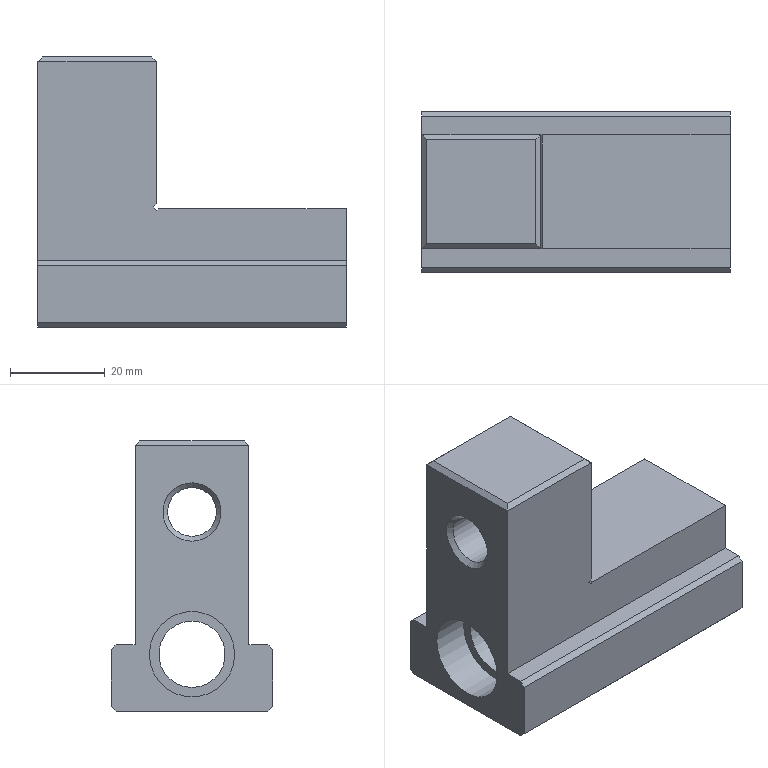Part | NX | features DATUM_CSYS 5, CHAMFER 4, SKETCH 4, BLOCK 3, CYLINDER 2, HOLE PACKAGE 2, SIMPLE HOLE 2, SYMBOLIC_THREAD 2, EXTRUDE 1 | 1 solid | 31 faces | box 65 x 34 x 57 mm | volume 53379 mm3 | plane 25 | cylinder 4 | cone 2 | commonest cylinder face diameters 18 x2 10.3 x1 14 x1
STEP:
#1=CARTESIAN_POINT('',(25.,5.,25.98));
#2=VERTEX_POINT('',#1);
#3=CARTESIAN_POINT('',(25.,5.,56.));
#4=VERTEX_POINT('',#3);
#5=CARTESIAN_POINT('',(25.,5.,0.));
#6=DIRECTION('',(0.,0.,1.));
#7=VECTOR('',#6,1000.);
#8=LINE('',#5,#7);
#9=EDGE_CURVE('',#2,#4,#8,.T.);
#10=ORIENTED_EDGE('',*,*,#9,.T.);
#11=CARTESIAN_POINT('',(0.,5.,56.));
#12=VERTEX_POINT('',#11);
#13=CARTESIAN_POINT('',(12.5,5.,56.));
#14=DIRECTION('',(-1.,0.,0.));
#15=VECTOR('',#14,1000.);
#16=LINE('',#13,#15);
#17=EDGE_CURVE('',#4,#12,#16,.T.);
#18=ORIENTED_EDGE('',*,*,#17,.T.);
#19=CARTESIAN_POINT('',(0.,5.,14.));
#20=VERTEX_POINT('',#19);
#21=CARTESIAN_POINT('',(0.,5.,0.));
#22=DIRECTION('',(0.,0.,1.));
#23=VECTOR('',#22,1000.);
#24=LINE('',#21,#23);
#25=EDGE_CURVE('',#20,#12,#24,.T.);
#26=ORIENTED_EDGE('',*,*,#25,.F.);
#27=CARTESIAN_POINT('',(65.,5.,14.));
#28=VERTEX_POINT('',#27);
#29=CARTESIAN_POINT('',(32.5,5.,14.));
#30=DIRECTION('',(1.,0.,0.));
#31=VECTOR('',#30,1000.);
#32=LINE('',#29,#31);
#33=EDGE_CURVE('',#20,#28,#32,.T.);
#34=ORIENTED_EDGE('',*,*,#33,.T.);
#35=CARTESIAN_POINT('',(65.,5.,25.));
#36=VERTEX_POINT('',#35);
#37=CARTESIAN_POINT('',(65.,5.,14.));
#38=DIRECTION('',(0.,0.,1.));
#39=VECTOR('',#38,1000.);
#40=LINE('',#37,#39);
#41=EDGE_CURVE('',#28,#36,#40,.T.);
#42=ORIENTED_EDGE('',*,*,#41,.T.);
#43=CARTESIAN_POINT('',(25.435,5.,25.));
#44=VERTEX_POINT('',#43);
#45=CARTESIAN_POINT('',(45.,5.,25.));
#46=DIRECTION('',(-1.,0.,0.));
#47=VECTOR('',#46,1000.);
#48=LINE('',#45,#47);
#49=EDGE_CURVE('',#36,#44,#48,.T.);
#50=ORIENTED_EDGE('',*,*,#49,.T.);
#51=CARTESIAN_POINT('',(25.081,5.,24.646));
#52=VERTEX_POINT('',#51);
#53=CARTESIAN_POINT('',(25.435,5.,25.));
#54=DIRECTION('',(-0.7071,0.,-0.7071));
#55=VECTOR('',#54,1000.);
#56=LINE('',#53,#55);
#57=EDGE_CURVE('',#44,#52,#56,.T.);
#58=ORIENTED_EDGE('',*,*,#57,.T.);
#59=CARTESIAN_POINT('',(24.374,5.,25.354));
#60=VERTEX_POINT('',#59);
#61=CARTESIAN_POINT('',(25.081,5.,24.646));
#62=DIRECTION('',(-0.7071,0.,0.7071));
#63=VECTOR('',#62,1000.);
#64=LINE('',#61,#63);
#65=EDGE_CURVE('',#52,#60,#64,.T.);
#66=ORIENTED_EDGE('',*,*,#65,.T.);
#67=CARTESIAN_POINT('',(24.374,5.,25.354));
#68=DIRECTION('',(0.7071,0.,0.7071));
#69=VECTOR('',#68,1000.);
#70=LINE('',#67,#69);
#71=EDGE_CURVE('',#60,#2,#70,.T.);
#72=ORIENTED_EDGE('',*,*,#71,.T.);
#73=EDGE_LOOP('',(#10,#18,#26,#34,#42,#50,#58,#66,#72));
#74=FACE_BOUND('',#73,.T.);
#75=CARTESIAN_POINT('',(12.5,5.,0.));
#76=DIRECTION('',(0.,-1.,0.));
#77=DIRECTION('',(0.,0.,-1.));
#78=AXIS2_PLACEMENT_3D('',#75,#76,#77);
#79=PLANE('',#78);
#80=ADVANCED_FACE('',(#74),#79,.T.);
#81=CARTESIAN_POINT('',(25.,17.,35.85));
#82=VERTEX_POINT('',#81);
#83=CARTESIAN_POINT('',(25.,17.,42.));
#84=DIRECTION('',(1.,0.,0.));
#85=DIRECTION('',(0.,0.,-1.));
#86=AXIS2_PLACEMENT_3D('',#83,#84,#85);
#87=CIRCLE('',#86,6.15);
#88=EDGE_CURVE('',#82,#82,#87,.F.);
#89=ORIENTED_EDGE('',*,*,#88,.T.);
#90=EDGE_LOOP('',(#89));
#91=FACE_BOUND('',#90,.T.);
#92=ORIENTED_EDGE('',*,*,#9,.F.);
#93=CARTESIAN_POINT('',(25.,29.,25.98));
#94=VERTEX_POINT('',#93);
#95=CARTESIAN_POINT('',(25.,29.,25.98));
#96=DIRECTION('',(0.,-1.,0.));
#97=VECTOR('',#96,1000.);
#98=LINE('',#95,#97);
#99=EDGE_CURVE('',#94,#2,#98,.T.);
#100=ORIENTED_EDGE('',*,*,#99,.F.);
#101=CARTESIAN_POINT('',(25.,29.,56.));
#102=VERTEX_POINT('',#101);
#103=CARTESIAN_POINT('',(25.,29.,0.));
#104=DIRECTION('',(0.,0.,1.));
#105=VECTOR('',#104,1000.);
#106=LINE('',#103,#105);
#107=EDGE_CURVE('',#94,#102,#106,.T.);
#108=ORIENTED_EDGE('',*,*,#107,.T.);
#109=CARTESIAN_POINT('',(25.,17.,56.));
#110=DIRECTION('',(0.,-1.,0.));
#111=VECTOR('',#110,1000.);
#112=LINE('',#109,#111);
#113=EDGE_CURVE('',#102,#4,#112,.T.);
#114=ORIENTED_EDGE('',*,*,#113,.T.);
#115=EDGE_LOOP('',(#92,#100,#108,#114));
#116=FACE_BOUND('',#115,.T.);
#117=CARTESIAN_POINT('',(25.,17.,0.));
#118=DIRECTION('',(1.,0.,0.));
#119=DIRECTION('',(0.,0.,-1.));
#120=AXIS2_PLACEMENT_3D('',#117,#118,#119);
#121=PLANE('',#120);
#122=ADVANCED_FACE('',(#91,#116),#121,.T.);
#123=CARTESIAN_POINT('',(25.435,29.,25.));
#124=VERTEX_POINT('',#123);
#125=CARTESIAN_POINT('',(65.,29.,25.));
#126=VERTEX_POINT('',#125);
#127=CARTESIAN_POINT('',(45.,29.,25.));
#128=DIRECTION('',(1.,0.,0.));
#129=VECTOR('',#128,1000.);
#130=LINE('',#127,#129);
#131=EDGE_CURVE('',#124,#126,#130,.T.);
#132=ORIENTED_EDGE('',*,*,#131,.F.);
#133=CARTESIAN_POINT('',(25.435,29.,25.));
#134=DIRECTION('',(0.,-1.,0.));
#135=VECTOR('',#134,1000.);
#136=LINE('',#133,#135);
#137=EDGE_CURVE('',#124,#44,#136,.T.);
#138=ORIENTED_EDGE('',*,*,#137,.T.);
#139=ORIENTED_EDGE('',*,*,#49,.F.);
#140=CARTESIAN_POINT('',(65.,17.,25.));
#141=DIRECTION('',(0.,-1.,0.));
#142=VECTOR('',#141,1000.);
#143=LINE('',#140,#142);
#144=EDGE_CURVE('',#126,#36,#143,.T.);
#145=ORIENTED_EDGE('',*,*,#144,.F.);
#146=EDGE_LOOP('',(#132,#138,#139,#145));
#147=FACE_BOUND('',#146,.T.);
#148=CARTESIAN_POINT('',(45.,17.,25.));
#149=DIRECTION('',(0.,0.,1.));
#150=DIRECTION('',(1.,0.,0.));
#151=AXIS2_PLACEMENT_3D('',#148,#149,#150);
#152=PLANE('',#151);
#153=ADVANCED_FACE('',(#147),#152,.T.);
#154=CARTESIAN_POINT('',(0.,1.,14.));
#155=VERTEX_POINT('',#154);
#156=CARTESIAN_POINT('',(0.,17.,14.));
#157=DIRECTION('',(0.,1.,0.));
#158=VECTOR('',#157,1000.);
#159=LINE('',#156,#158);
#160=EDGE_CURVE('',#155,#20,#159,.T.);
#161=ORIENTED_EDGE('',*,*,#160,.F.);
#162=CARTESIAN_POINT('',(65.,1.,14.));
#163=VERTEX_POINT('',#162);
#164=CARTESIAN_POINT('',(32.5,1.,14.));
#165=DIRECTION('',(1.,0.,0.));
#166=VECTOR('',#165,1000.);
#167=LINE('',#164,#166);
#168=EDGE_CURVE('',#155,#163,#167,.T.);
#169=ORIENTED_EDGE('',*,*,#168,.T.);
#170=CARTESIAN_POINT('',(65.,17.,14.));
#171=DIRECTION('',(0.,-1.,0.));
#172=VECTOR('',#171,1000.);
#173=LINE('',#170,#172);
#174=EDGE_CURVE('',#28,#163,#173,.T.);
#175=ORIENTED_EDGE('',*,*,#174,.F.);
#176=ORIENTED_EDGE('',*,*,#33,.F.);
#177=EDGE_LOOP('',(#161,#169,#175,#176));
#178=FACE_BOUND('',#177,.T.);
#179=CARTESIAN_POINT('',(32.5,17.,14.));
#180=DIRECTION('',(0.,0.,1.));
#181=DIRECTION('',(1.,0.,0.));
#182=AXIS2_PLACEMENT_3D('',#179,#180,#181);
#183=PLANE('',#182);
#184=ADVANCED_FACE('',(#178),#183,.T.);
#185=CARTESIAN_POINT('',(65.,33.,14.));
#186=VERTEX_POINT('',#185);
#187=CARTESIAN_POINT('',(65.,29.,14.));
#188=VERTEX_POINT('',#187);
#189=CARTESIAN_POINT('',(65.,17.,14.));
#190=DIRECTION('',(0.,-1.,0.));
#191=VECTOR('',#190,1000.);
#192=LINE('',#189,#191);
#193=EDGE_CURVE('',#186,#188,#192,.T.);
#194=ORIENTED_EDGE('',*,*,#193,.F.);
#195=CARTESIAN_POINT('',(0.,33.,14.));
#196=VERTEX_POINT('',#195);
#197=CARTESIAN_POINT('',(32.5,33.,14.));
#198=DIRECTION('',(-1.,0.,0.));
#199=VECTOR('',#198,1000.);
#200=LINE('',#197,#199);
#201=EDGE_CURVE('',#186,#196,#200,.T.);
#202=ORIENTED_EDGE('',*,*,#201,.T.);
#203=CARTESIAN_POINT('',(0.,29.,14.));
#204=VERTEX_POINT('',#203);
#205=CARTESIAN_POINT('',(0.,17.,14.));
#206=DIRECTION('',(0.,1.,0.));
#207=VECTOR('',#206,1000.);
#208=LINE('',#205,#207);
#209=EDGE_CURVE('',#204,#196,#208,.T.);
#210=ORIENTED_EDGE('',*,*,#209,.F.);
#211=CARTESIAN_POINT('',(32.5,29.,14.));
#212=DIRECTION('',(-1.,0.,0.));
#213=VECTOR('',#212,1000.);
#214=LINE('',#211,#213);
#215=EDGE_CURVE('',#188,#204,#214,.T.);
#216=ORIENTED_EDGE('',*,*,#215,.F.);
#217=EDGE_LOOP('',(#194,#202,#210,#216));
#218=FACE_BOUND('',#217,.T.);
#219=CARTESIAN_POINT('',(32.5,17.,14.));
#220=DIRECTION('',(0.,0.,1.));
#221=DIRECTION('',(1.,0.,0.));
#222=AXIS2_PLACEMENT_3D('',#219,#220,#221);
#223=PLANE('',#222);
#224=ADVANCED_FACE('',(#218),#223,.T.);
#225=CARTESIAN_POINT('',(65.,0.,1.));
#226=VERTEX_POINT('',#225);
#227=CARTESIAN_POINT('',(65.,0.,13.));
#228=VERTEX_POINT('',#227);
#229=CARTESIAN_POINT('',(65.,0.,0.));
#230=DIRECTION('',(0.,0.,1.));
#231=VECTOR('',#230,1000.);
#232=LINE('',#229,#231);
#233=EDGE_CURVE('',#226,#228,#232,.T.);
#234=ORIENTED_EDGE('',*,*,#233,.T.);
#235=CARTESIAN_POINT('',(0.,0.,13.));
#236=VERTEX_POINT('',#235);
#237=CARTESIAN_POINT('',(32.5,0.,13.));
#238=DIRECTION('',(-1.,0.,0.));
#239=VECTOR('',#238,1000.);
#240=LINE('',#237,#239);
#241=EDGE_CURVE('',#228,#236,#240,.T.);
#242=ORIENTED_EDGE('',*,*,#241,.T.);
#243=CARTESIAN_POINT('',(0.,0.,1.));
#244=VERTEX_POINT('',#243);
#245=CARTESIAN_POINT('',(0.,0.,0.));
#246=DIRECTION('',(0.,0.,1.));
#247=VECTOR('',#246,1000.);
#248=LINE('',#245,#247);
#249=EDGE_CURVE('',#244,#236,#248,.T.);
#250=ORIENTED_EDGE('',*,*,#249,.F.);
#251=CARTESIAN_POINT('',(32.5,0.,1.));
#252=DIRECTION('',(1.,0.,0.));
#253=VECTOR('',#252,1000.);
#254=LINE('',#251,#253);
#255=EDGE_CURVE('',#244,#226,#254,.T.);
#256=ORIENTED_EDGE('',*,*,#255,.T.);
#257=EDGE_LOOP('',(#234,#242,#250,#256));
#258=FACE_BOUND('',#257,.T.);
#259=CARTESIAN_POINT('',(32.5,0.,0.));
#260=DIRECTION('',(0.,-1.,0.));
#261=DIRECTION('',(0.,0.,-1.));
#262=AXIS2_PLACEMENT_3D('',#259,#260,#261);
#263=PLANE('',#262);
#264=ADVANCED_FACE('',(#258),#263,.T.);
#265=CARTESIAN_POINT('',(0.,17.,48.15));
#266=VERTEX_POINT('',#265);
#267=CARTESIAN_POINT('',(0.,17.,42.));
#268=DIRECTION('',(-1.,0.,0.));
#269=DIRECTION('',(0.,0.,1.));
#270=AXIS2_PLACEMENT_3D('',#267,#268,#269);
#271=CIRCLE('',#270,6.15);
#272=EDGE_CURVE('',#266,#266,#271,.F.);
#273=ORIENTED_EDGE('',*,*,#272,.T.);
#274=EDGE_LOOP('',(#273));
#275=FACE_BOUND('',#274,.T.);
#276=CARTESIAN_POINT('',(0.,26.,12.));
#277=VERTEX_POINT('',#276);
#278=CARTESIAN_POINT('',(0.,17.,12.));
#279=DIRECTION('',(1.,0.,0.));
#280=DIRECTION('',(0.,1.,0.));
#281=AXIS2_PLACEMENT_3D('',#278,#279,#280);
#282=CIRCLE('',#281,9.);
#283=EDGE_CURVE('',#277,#277,#282,.T.);
#284=ORIENTED_EDGE('',*,*,#283,.T.);
#285=EDGE_LOOP('',(#284));
#286=FACE_BOUND('',#285,.T.);
#287=CARTESIAN_POINT('',(0.,34.,1.));
#288=VERTEX_POINT('',#287);
#289=CARTESIAN_POINT('',(0.,34.,13.));
#290=VERTEX_POINT('',#289);
#291=CARTESIAN_POINT('',(0.,34.,0.));
#292=DIRECTION('',(0.,0.,1.));
#293=VECTOR('',#292,1000.);
#294=LINE('',#291,#293);
#295=EDGE_CURVE('',#288,#290,#294,.T.);
#296=ORIENTED_EDGE('',*,*,#295,.F.);
#297=CARTESIAN_POINT('',(0.,33.,0.));
#298=VERTEX_POINT('',#297);
#299=CARTESIAN_POINT('',(0.,25.,-8.));
#300=DIRECTION('',(0.,0.7071,0.7071));
#301=VECTOR('',#300,1000.);
#302=LINE('',#299,#301);
#303=EDGE_CURVE('',#288,#298,#302,.F.);
#304=ORIENTED_EDGE('',*,*,#303,.T.);
#305=CARTESIAN_POINT('',(0.,1.,0.));
#306=VERTEX_POINT('',#305);
#307=CARTESIAN_POINT('',(0.,17.,0.));
#308=DIRECTION('',(0.,-1.,0.));
#309=VECTOR('',#308,1000.);
#310=LINE('',#307,#309);
#311=EDGE_CURVE('',#298,#306,#310,.T.);
#312=ORIENTED_EDGE('',*,*,#311,.T.);
#313=CARTESIAN_POINT('',(0.,9.,-8.));
#314=DIRECTION('',(0.,0.7071,-0.7071));
#315=VECTOR('',#314,1000.);
#316=LINE('',#313,#315);
#317=EDGE_CURVE('',#306,#244,#316,.F.);
#318=ORIENTED_EDGE('',*,*,#317,.T.);
#319=ORIENTED_EDGE('',*,*,#249,.T.);
#320=CARTESIAN_POINT('',(0.,2.,15.));
#321=DIRECTION('',(0.,-0.7071,-0.7071));
#322=VECTOR('',#321,1000.);
#323=LINE('',#320,#322);
#324=EDGE_CURVE('',#236,#155,#323,.F.);
#325=ORIENTED_EDGE('',*,*,#324,.T.);
#326=ORIENTED_EDGE('',*,*,#160,.T.);
#327=ORIENTED_EDGE('',*,*,#25,.T.);
#328=CARTESIAN_POINT('',(0.,29.,56.));
#329=VERTEX_POINT('',#328);
#330=CARTESIAN_POINT('',(0.,17.,56.));
#331=DIRECTION('',(0.,1.,0.));
#332=VECTOR('',#331,1000.);
#333=LINE('',#330,#332);
#334=EDGE_CURVE('',#12,#329,#333,.T.);
#335=ORIENTED_EDGE('',*,*,#334,.T.);
#336=CARTESIAN_POINT('',(0.,29.,0.));
#337=DIRECTION('',(0.,0.,1.));
#338=VECTOR('',#337,1000.);
#339=LINE('',#336,#338);
#340=EDGE_CURVE('',#204,#329,#339,.T.);
#341=ORIENTED_EDGE('',*,*,#340,.F.);
#342=ORIENTED_EDGE('',*,*,#209,.T.);
#343=CARTESIAN_POINT('',(0.,32.,15.));
#344=DIRECTION('',(0.,-0.7071,0.7071));
#345=VECTOR('',#344,1000.);
#346=LINE('',#343,#345);
#347=EDGE_CURVE('',#196,#290,#346,.F.);
#348=ORIENTED_EDGE('',*,*,#347,.T.);
#349=EDGE_LOOP('',(#296,#304,#312,#318,#319,#325,#326,#327,#335,#341,#342,#348));
#350=FACE_BOUND('',#349,.T.);
#351=CARTESIAN_POINT('',(0.,17.,0.));
#352=DIRECTION('',(-1.,0.,0.));
#353=DIRECTION('',(0.,0.,1.));
#354=AXIS2_PLACEMENT_3D('',#351,#352,#353);
#355=PLANE('',#354);
#356=ADVANCED_FACE('',(#275,#286,#350),#355,.T.);
#357=CARTESIAN_POINT('',(65.,34.,1.));
#358=VERTEX_POINT('',#357);
#359=CARTESIAN_POINT('',(65.,34.,13.));
#360=VERTEX_POINT('',#359);
#361=CARTESIAN_POINT('',(65.,34.,0.));
#362=DIRECTION('',(0.,0.,1.));
#363=VECTOR('',#362,1000.);
#364=LINE('',#361,#363);
#365=EDGE_CURVE('',#358,#360,#364,.T.);
#366=ORIENTED_EDGE('',*,*,#365,.F.);
#367=CARTESIAN_POINT('',(32.5,34.,1.));
#368=DIRECTION('',(-1.,0.,0.));
#369=VECTOR('',#368,1000.);
#370=LINE('',#367,#369);
#371=EDGE_CURVE('',#358,#288,#370,.T.);
#372=ORIENTED_EDGE('',*,*,#371,.T.);
#373=ORIENTED_EDGE('',*,*,#295,.T.);
#374=CARTESIAN_POINT('',(32.5,34.,13.));
#375=DIRECTION('',(1.,0.,0.));
#376=VECTOR('',#375,1000.);
#377=LINE('',#374,#376);
#378=EDGE_CURVE('',#290,#360,#377,.T.);
#379=ORIENTED_EDGE('',*,*,#378,.T.);
#380=EDGE_LOOP('',(#366,#372,#373,#379));
#381=FACE_BOUND('',#380,.T.);
#382=CARTESIAN_POINT('',(32.5,34.,0.));
#383=DIRECTION('',(0.,1.,0.));
#384=DIRECTION('',(0.,0.,1.));
#385=AXIS2_PLACEMENT_3D('',#382,#383,#384);
#386=PLANE('',#385);
#387=ADVANCED_FACE('',(#381),#386,.T.);
#388=ORIENTED_EDGE('',*,*,#311,.F.);
#389=CARTESIAN_POINT('',(65.,33.,0.));
#390=VERTEX_POINT('',#389);
#391=CARTESIAN_POINT('',(32.5,33.,0.));
#392=DIRECTION('',(1.,0.,0.));
#393=VECTOR('',#392,1000.);
#394=LINE('',#391,#393);
#395=EDGE_CURVE('',#298,#390,#394,.T.);
#396=ORIENTED_EDGE('',*,*,#395,.T.);
#397=CARTESIAN_POINT('',(65.,1.,0.));
#398=VERTEX_POINT('',#397);
#399=CARTESIAN_POINT('',(65.,17.,0.));
#400=DIRECTION('',(0.,1.,0.));
#401=VECTOR('',#400,1000.);
#402=LINE('',#399,#401);
#403=EDGE_CURVE('',#398,#390,#402,.T.);
#404=ORIENTED_EDGE('',*,*,#403,.F.);
#405=CARTESIAN_POINT('',(32.5,1.,0.));
#406=DIRECTION('',(-1.,0.,0.));
#407=VECTOR('',#406,1000.);
#408=LINE('',#405,#407);
#409=EDGE_CURVE('',#398,#306,#408,.T.);
#410=ORIENTED_EDGE('',*,*,#409,.T.);
#411=EDGE_LOOP('',(#388,#396,#404,#410));
#412=FACE_BOUND('',#411,.T.);
#413=CARTESIAN_POINT('',(32.5,17.,0.));
#414=DIRECTION('',(0.,0.,-1.));
#415=DIRECTION('',(-1.,0.,0.));
#416=AXIS2_PLACEMENT_3D('',#413,#414,#415);
#417=PLANE('',#416);
#418=ADVANCED_FACE('',(#412),#417,.T.);
#419=CARTESIAN_POINT('',(65.,8.,12.));
#420=VERTEX_POINT('',#419);
#421=CARTESIAN_POINT('',(65.,17.,12.));
#422=DIRECTION('',(-1.,0.,0.));
#423=DIRECTION('',(0.,-1.,0.));
#424=AXIS2_PLACEMENT_3D('',#421,#422,#423);
#425=CIRCLE('',#424,9.);
#426=EDGE_CURVE('',#420,#420,#425,.T.);
#427=ORIENTED_EDGE('',*,*,#426,.T.);
#428=EDGE_LOOP('',(#427));
#429=FACE_BOUND('',#428,.T.);
#430=ORIENTED_EDGE('',*,*,#403,.T.);
#431=CARTESIAN_POINT('',(65.,25.,-8.));
#432=DIRECTION('',(0.,-0.7071,-0.7071));
#433=VECTOR('',#432,1000.);
#434=LINE('',#431,#433);
#435=EDGE_CURVE('',#390,#358,#434,.F.);
#436=ORIENTED_EDGE('',*,*,#435,.T.);
#437=ORIENTED_EDGE('',*,*,#365,.T.);
#438=CARTESIAN_POINT('',(65.,32.,15.));
#439=DIRECTION('',(0.,0.7071,-0.7071));
#440=VECTOR('',#439,1000.);
#441=LINE('',#438,#440);
#442=EDGE_CURVE('',#360,#186,#441,.F.);
#443=ORIENTED_EDGE('',*,*,#442,.T.);
#444=ORIENTED_EDGE('',*,*,#193,.T.);
#445=CARTESIAN_POINT('',(65.,29.,14.));
#446=DIRECTION('',(0.,0.,1.));
#447=VECTOR('',#446,1000.);
#448=LINE('',#445,#447);
#449=EDGE_CURVE('',#188,#126,#448,.T.);
#450=ORIENTED_EDGE('',*,*,#449,.T.);
#451=ORIENTED_EDGE('',*,*,#144,.T.);
#452=ORIENTED_EDGE('',*,*,#41,.F.);
#453=ORIENTED_EDGE('',*,*,#174,.T.);
#454=CARTESIAN_POINT('',(65.,2.,15.));
#455=DIRECTION('',(0.,0.7071,0.7071));
#456=VECTOR('',#455,1000.);
#457=LINE('',#454,#456);
#458=EDGE_CURVE('',#163,#228,#457,.F.);
#459=ORIENTED_EDGE('',*,*,#458,.T.);
#460=ORIENTED_EDGE('',*,*,#233,.F.);
#461=CARTESIAN_POINT('',(65.,9.,-8.));
#462=DIRECTION('',(0.,-0.7071,0.7071));
#463=VECTOR('',#462,1000.);
#464=LINE('',#461,#463);
#465=EDGE_CURVE('',#226,#398,#464,.F.);
#466=ORIENTED_EDGE('',*,*,#465,.T.);
#467=EDGE_LOOP('',(#430,#436,#437,#443,#444,#450,#451,#452,#453,#459,#460,#466));
#468=FACE_BOUND('',#467,.T.);
#469=CARTESIAN_POINT('',(65.,17.,0.));
#470=DIRECTION('',(1.,0.,0.));
#471=DIRECTION('',(0.,0.,-1.));
#472=AXIS2_PLACEMENT_3D('',#469,#470,#471);
#473=PLANE('',#472);
#474=ADVANCED_FACE('',(#429,#468),#473,.T.);
#475=CARTESIAN_POINT('',(24.,6.,57.));
#476=VERTEX_POINT('',#475);
#477=CARTESIAN_POINT('',(24.,28.,57.));
#478=VERTEX_POINT('',#477);
#479=CARTESIAN_POINT('',(24.,17.,57.));
#480=DIRECTION('',(0.,1.,0.));
#481=VECTOR('',#480,1000.);
#482=LINE('',#479,#481);
#483=EDGE_CURVE('',#476,#478,#482,.T.);
#484=ORIENTED_EDGE('',*,*,#483,.T.);
#485=CARTESIAN_POINT('',(1.,28.,57.));
#486=VERTEX_POINT('',#485);
#487=CARTESIAN_POINT('',(12.5,28.,57.));
#488=DIRECTION('',(-1.,0.,0.));
#489=VECTOR('',#488,1000.);
#490=LINE('',#487,#489);
#491=EDGE_CURVE('',#478,#486,#490,.T.);
#492=ORIENTED_EDGE('',*,*,#491,.T.);
#493=CARTESIAN_POINT('',(1.,6.,57.));
#494=VERTEX_POINT('',#493);
#495=CARTESIAN_POINT('',(1.,17.,57.));
#496=DIRECTION('',(0.,-1.,0.));
#497=VECTOR('',#496,1000.);
#498=LINE('',#495,#497);
#499=EDGE_CURVE('',#486,#494,#498,.T.);
#500=ORIENTED_EDGE('',*,*,#499,.T.);
#501=CARTESIAN_POINT('',(12.5,6.,57.));
#502=DIRECTION('',(1.,0.,0.));
#503=VECTOR('',#502,1000.);
#504=LINE('',#501,#503);
#505=EDGE_CURVE('',#494,#476,#504,.T.);
#506=ORIENTED_EDGE('',*,*,#505,.T.);
#507=EDGE_LOOP('',(#484,#492,#500,#506));
#508=FACE_BOUND('',#507,.T.);
#509=CARTESIAN_POINT('',(12.5,17.,57.));
#510=DIRECTION('',(0.,0.,1.));
#511=DIRECTION('',(1.,0.,0.));
#512=AXIS2_PLACEMENT_3D('',#509,#510,#511);
#513=PLANE('',#512);
#514=ADVANCED_FACE('',(#508),#513,.T.);
#515=ORIENTED_EDGE('',*,*,#340,.T.);
#516=CARTESIAN_POINT('',(12.5,29.,56.));
#517=DIRECTION('',(1.,0.,0.));
#518=VECTOR('',#517,1000.);
#519=LINE('',#516,#518);
#520=EDGE_CURVE('',#329,#102,#519,.T.);
#521=ORIENTED_EDGE('',*,*,#520,.T.);
#522=ORIENTED_EDGE('',*,*,#107,.F.);
#523=CARTESIAN_POINT('',(24.374,29.,25.354));
#524=VERTEX_POINT('',#523);
#525=CARTESIAN_POINT('',(24.374,29.,25.354));
#526=DIRECTION('',(0.7071,0.,0.7071));
#527=VECTOR('',#526,1000.);
#528=LINE('',#525,#527);
#529=EDGE_CURVE('',#524,#94,#528,.T.);
#530=ORIENTED_EDGE('',*,*,#529,.F.);
#531=CARTESIAN_POINT('',(25.081,29.,24.646));
#532=VERTEX_POINT('',#531);
#533=CARTESIAN_POINT('',(25.081,29.,24.646));
#534=DIRECTION('',(-0.7071,0.,0.7071));
#535=VECTOR('',#534,1000.);
#536=LINE('',#533,#535);
#537=EDGE_CURVE('',#532,#524,#536,.T.);
#538=ORIENTED_EDGE('',*,*,#537,.F.);
#539=CARTESIAN_POINT('',(25.435,29.,25.));
#540=DIRECTION('',(-0.7071,0.,-0.7071));
#541=VECTOR('',#540,1000.);
#542=LINE('',#539,#541);
#543=EDGE_CURVE('',#124,#532,#542,.T.);
#544=ORIENTED_EDGE('',*,*,#543,.F.);
#545=ORIENTED_EDGE('',*,*,#131,.T.);
#546=ORIENTED_EDGE('',*,*,#449,.F.);
#547=ORIENTED_EDGE('',*,*,#215,.T.);
#548=EDGE_LOOP('',(#515,#521,#522,#530,#538,#544,#545,#546,#547));
#549=FACE_BOUND('',#548,.T.);
#550=CARTESIAN_POINT('',(12.5,29.,0.));
#551=DIRECTION('',(0.,1.,0.));
#552=DIRECTION('',(0.,0.,1.));
#553=AXIS2_PLACEMENT_3D('',#550,#551,#552);
#554=PLANE('',#553);
#555=ADVANCED_FACE('',(#549),#554,.T.);
#556=CARTESIAN_POINT('',(8.,17.,5.));
#557=VERTEX_POINT('',#556);
#558=CARTESIAN_POINT('',(8.,17.,12.));
#559=DIRECTION('',(1.,0.,0.));
#560=DIRECTION('',(0.,0.,-1.));
#561=AXIS2_PLACEMENT_3D('',#558,#559,#560);
#562=CIRCLE('',#561,7.);
#563=EDGE_CURVE('',#557,#557,#562,.T.);
#564=ORIENTED_EDGE('',*,*,#563,.T.);
#565=EDGE_LOOP('',(#564));
#566=FACE_BOUND('',#565,.T.);
#567=CARTESIAN_POINT('',(8.,26.,12.));
#568=VERTEX_POINT('',#567);
#569=CARTESIAN_POINT('',(8.,17.,12.));
#570=DIRECTION('',(-1.,0.,0.));
#571=DIRECTION('',(0.,1.,0.));
#572=AXIS2_PLACEMENT_3D('',#569,#570,#571);
#573=CIRCLE('',#572,9.);
#574=EDGE_CURVE('',#568,#568,#573,.F.);
#575=ORIENTED_EDGE('',*,*,#574,.F.);
#576=EDGE_LOOP('',(#575));
#577=FACE_BOUND('',#576,.T.);
#578=CARTESIAN_POINT('',(8.,17.,12.));
#579=DIRECTION('',(1.,0.,0.));
#580=DIRECTION('',(0.,0.,-1.));
#581=AXIS2_PLACEMENT_3D('',#578,#579,#580);
#582=PLANE('',#581);
#583=ADVANCED_FACE('',(#566,#577),#582,.F.);
#584=ORIENTED_EDGE('',*,*,#574,.T.);
#585=EDGE_LOOP('',(#584));
#586=FACE_BOUND('',#585,.T.);
#587=ORIENTED_EDGE('',*,*,#283,.F.);
#588=EDGE_LOOP('',(#587));
#589=FACE_BOUND('',#588,.T.);
#590=CARTESIAN_POINT('',(0.,17.,12.));
#591=DIRECTION('',(1.,0.,0.));
#592=DIRECTION('',(0.,1.,0.));
#593=AXIS2_PLACEMENT_3D('',#590,#591,#592);
#594=CYLINDRICAL_SURFACE('',#593,9.);
#595=ADVANCED_FACE('',(#586,#589),#594,.F.);
#596=CARTESIAN_POINT('',(57.,17.,5.));
#597=VERTEX_POINT('',#596);
#598=CARTESIAN_POINT('',(57.,17.,12.));
#599=DIRECTION('',(1.,0.,0.));
#600=DIRECTION('',(0.,0.,-1.));
#601=AXIS2_PLACEMENT_3D('',#598,#599,#600);
#602=CIRCLE('',#601,7.);
#603=EDGE_CURVE('',#597,#597,#602,.T.);
#604=ORIENTED_EDGE('',*,*,#603,.F.);
#605=EDGE_LOOP('',(#604));
#606=FACE_BOUND('',#605,.T.);
#607=CARTESIAN_POINT('',(57.,8.,12.));
#608=VERTEX_POINT('',#607);
#609=CARTESIAN_POINT('',(57.,17.,12.));
#610=DIRECTION('',(1.,0.,0.));
#611=DIRECTION('',(0.,-1.,0.));
#612=AXIS2_PLACEMENT_3D('',#609,#610,#611);
#613=CIRCLE('',#612,9.);
#614=EDGE_CURVE('',#608,#608,#613,.F.);
#615=ORIENTED_EDGE('',*,*,#614,.F.);
#616=EDGE_LOOP('',(#615));
#617=FACE_BOUND('',#616,.T.);
#618=CARTESIAN_POINT('',(57.,17.,12.));
#619=DIRECTION('',(-1.,0.,0.));
#620=DIRECTION('',(0.,0.,1.));
#621=AXIS2_PLACEMENT_3D('',#618,#619,#620);
#622=PLANE('',#621);
#623=ADVANCED_FACE('',(#606,#617),#622,.F.);
#624=ORIENTED_EDGE('',*,*,#614,.T.);
#625=EDGE_LOOP('',(#624));
#626=FACE_BOUND('',#625,.T.);
#627=ORIENTED_EDGE('',*,*,#426,.F.);
#628=EDGE_LOOP('',(#627));
#629=FACE_BOUND('',#628,.T.);
#630=CARTESIAN_POINT('',(65.,17.,12.));
#631=DIRECTION('',(-1.,0.,0.));
#632=DIRECTION('',(0.,-1.,0.));
#633=AXIS2_PLACEMENT_3D('',#630,#631,#632);
#634=CYLINDRICAL_SURFACE('',#633,9.);
#635=ADVANCED_FACE('',(#626,#629),#634,.F.);
#636=ORIENTED_EDGE('',*,*,#603,.T.);
#637=EDGE_LOOP('',(#636));
#638=FACE_BOUND('',#637,.T.);
#639=ORIENTED_EDGE('',*,*,#563,.F.);
#640=EDGE_LOOP('',(#639));
#641=FACE_BOUND('',#640,.T.);
#642=CARTESIAN_POINT('',(8.,17.,12.));
#643=DIRECTION('',(1.,0.,0.));
#644=DIRECTION('',(0.,0.,-1.));
#645=AXIS2_PLACEMENT_3D('',#642,#643,#644);
#646=CYLINDRICAL_SURFACE('',#645,7.);
#647=ADVANCED_FACE('',(#638,#641),#646,.F.);
#648=CARTESIAN_POINT('',(24.,17.,36.85));
#649=VERTEX_POINT('',#648);
#650=CARTESIAN_POINT('',(24.,17.,42.));
#651=DIRECTION('',(1.,0.,0.));
#652=DIRECTION('',(0.,0.,-1.));
#653=AXIS2_PLACEMENT_3D('',#650,#651,#652);
#654=CIRCLE('',#653,5.15);
#655=EDGE_CURVE('',#649,#649,#654,.T.);
#656=ORIENTED_EDGE('',*,*,#655,.T.);
#657=EDGE_LOOP('',(#656));
#658=FACE_BOUND('',#657,.T.);
#659=CARTESIAN_POINT('',(1.,17.,47.15));
#660=VERTEX_POINT('',#659);
#661=CARTESIAN_POINT('',(1.,17.,42.));
#662=DIRECTION('',(-1.,0.,0.));
#663=DIRECTION('',(0.,0.,1.));
#664=AXIS2_PLACEMENT_3D('',#661,#662,#663);
#665=CIRCLE('',#664,5.15);
#666=EDGE_CURVE('',#660,#660,#665,.T.);
#667=ORIENTED_EDGE('',*,*,#666,.T.);
#668=EDGE_LOOP('',(#667));
#669=FACE_BOUND('',#668,.T.);
#670=CARTESIAN_POINT('',(0.,17.,42.));
#671=DIRECTION('',(1.,0.,0.));
#672=DIRECTION('',(0.,0.,-1.));
#673=AXIS2_PLACEMENT_3D('',#670,#671,#672);
#674=CYLINDRICAL_SURFACE('',#673,5.15);
#675=ADVANCED_FACE('',(#658,#669),#674,.F.);
#676=ORIENTED_EDGE('',*,*,#499,.F.);
#677=CARTESIAN_POINT('',(4.,25.,60.));
#678=DIRECTION('',(-0.5774,0.5774,-0.5774));
#679=VECTOR('',#678,1000.);
#680=LINE('',#677,#679);
#681=EDGE_CURVE('',#486,#329,#680,.T.);
#682=ORIENTED_EDGE('',*,*,#681,.T.);
#683=ORIENTED_EDGE('',*,*,#334,.F.);
#684=CARTESIAN_POINT('',(4.,9.,60.));
#685=DIRECTION('',(0.5774,0.5774,0.5774));
#686=VECTOR('',#685,1000.);
#687=LINE('',#684,#686);
#688=EDGE_CURVE('',#12,#494,#687,.T.);
#689=ORIENTED_EDGE('',*,*,#688,.T.);
#690=EDGE_LOOP('',(#676,#682,#683,#689));
#691=FACE_BOUND('',#690,.T.);
#692=CARTESIAN_POINT('',(0.,17.,56.));
#693=DIRECTION('',(0.7071,0.,-0.7071));
#694=DIRECTION('',(0.,1.,0.));
#695=AXIS2_PLACEMENT_3D('',#692,#693,#694);
#696=PLANE('',#695);
#697=ADVANCED_FACE('',(#691),#696,.F.);
#698=ORIENTED_EDGE('',*,*,#113,.F.);
#699=CARTESIAN_POINT('',(21.,25.,60.));
#700=DIRECTION('',(-0.5774,-0.5774,0.5774));
#701=VECTOR('',#700,1000.);
#702=LINE('',#699,#701);
#703=EDGE_CURVE('',#102,#478,#702,.T.);
#704=ORIENTED_EDGE('',*,*,#703,.T.);
#705=ORIENTED_EDGE('',*,*,#483,.F.);
#706=CARTESIAN_POINT('',(21.,9.,60.));
#707=DIRECTION('',(0.5774,-0.5774,-0.5774));
#708=VECTOR('',#707,1000.);
#709=LINE('',#706,#708);
#710=EDGE_CURVE('',#476,#4,#709,.T.);
#711=ORIENTED_EDGE('',*,*,#710,.T.);
#712=EDGE_LOOP('',(#698,#704,#705,#711));
#713=FACE_BOUND('',#712,.T.);
#714=CARTESIAN_POINT('',(25.,17.,56.));
#715=DIRECTION('',(-0.7071,0.,-0.7071));
#716=DIRECTION('',(0.,-1.,0.));
#717=AXIS2_PLACEMENT_3D('',#714,#715,#716);
#718=PLANE('',#717);
#719=ADVANCED_FACE('',(#713),#718,.F.);
#720=ORIENTED_EDGE('',*,*,#88,.F.);
#721=EDGE_LOOP('',(#720));
#722=FACE_BOUND('',#721,.T.);
#723=ORIENTED_EDGE('',*,*,#655,.F.);
#724=EDGE_LOOP('',(#723));
#725=FACE_BOUND('',#724,.T.);
#726=CARTESIAN_POINT('',(24.,17.,42.));
#727=DIRECTION('',(1.,0.,0.));
#728=DIRECTION('',(0.,0.,-1.));
#729=AXIS2_PLACEMENT_3D('',#726,#727,#728);
#730=CONICAL_SURFACE('',#729,5.15,0.7854);
#731=ADVANCED_FACE('',(#722,#725),#730,.F.);
#732=ORIENTED_EDGE('',*,*,#666,.F.);
#733=EDGE_LOOP('',(#732));
#734=FACE_BOUND('',#733,.T.);
#735=ORIENTED_EDGE('',*,*,#272,.F.);
#736=EDGE_LOOP('',(#735));
#737=FACE_BOUND('',#736,.T.);
#738=CARTESIAN_POINT('',(0.,17.,42.));
#739=DIRECTION('',(-1.,0.,0.));
#740=DIRECTION('',(0.,0.,1.));
#741=AXIS2_PLACEMENT_3D('',#738,#739,#740);
#742=CONICAL_SURFACE('',#741,6.15,0.7854);
#743=ADVANCED_FACE('',(#734,#737),#742,.F.);
#744=ORIENTED_EDGE('',*,*,#435,.F.);
#745=ORIENTED_EDGE('',*,*,#395,.F.);
#746=ORIENTED_EDGE('',*,*,#303,.F.);
#747=ORIENTED_EDGE('',*,*,#371,.F.);
#748=EDGE_LOOP('',(#744,#745,#746,#747));
#749=FACE_BOUND('',#748,.T.);
#750=CARTESIAN_POINT('',(32.5,34.,1.));
#751=DIRECTION('',(0.,-0.7071,0.7071));
#752=DIRECTION('',(-1.,0.,0.));
#753=AXIS2_PLACEMENT_3D('',#750,#751,#752);
#754=PLANE('',#753);
#755=ADVANCED_FACE('',(#749),#754,.F.);
#756=ORIENTED_EDGE('',*,*,#347,.F.);
#757=ORIENTED_EDGE('',*,*,#201,.F.);
#758=ORIENTED_EDGE('',*,*,#442,.F.);
#759=ORIENTED_EDGE('',*,*,#378,.F.);
#760=EDGE_LOOP('',(#756,#757,#758,#759));
#761=FACE_BOUND('',#760,.T.);
#762=CARTESIAN_POINT('',(32.5,34.,13.));
#763=DIRECTION('',(0.,-0.7071,-0.7071));
#764=DIRECTION('',(1.,0.,0.));
#765=AXIS2_PLACEMENT_3D('',#762,#763,#764);
#766=PLANE('',#765);
#767=ADVANCED_FACE('',(#761),#766,.F.);
#768=ORIENTED_EDGE('',*,*,#458,.F.);
#769=ORIENTED_EDGE('',*,*,#168,.F.);
#770=ORIENTED_EDGE('',*,*,#324,.F.);
#771=ORIENTED_EDGE('',*,*,#241,.F.);
#772=EDGE_LOOP('',(#768,#769,#770,#771));
#773=FACE_BOUND('',#772,.T.);
#774=CARTESIAN_POINT('',(32.5,0.,13.));
#775=DIRECTION('',(0.,0.7071,-0.7071));
#776=DIRECTION('',(-1.,0.,0.));
#777=AXIS2_PLACEMENT_3D('',#774,#775,#776);
#778=PLANE('',#777);
#779=ADVANCED_FACE('',(#773),#778,.F.);
#780=ORIENTED_EDGE('',*,*,#317,.F.);
#781=ORIENTED_EDGE('',*,*,#409,.F.);
#782=ORIENTED_EDGE('',*,*,#465,.F.);
#783=ORIENTED_EDGE('',*,*,#255,.F.);
#784=EDGE_LOOP('',(#780,#781,#782,#783));
#785=FACE_BOUND('',#784,.T.);
#786=CARTESIAN_POINT('',(32.5,0.,1.));
#787=DIRECTION('',(0.,0.7071,0.7071));
#788=DIRECTION('',(1.,0.,0.));
#789=AXIS2_PLACEMENT_3D('',#786,#787,#788);
#790=PLANE('',#789);
#791=ADVANCED_FACE('',(#785),#790,.F.);
#792=ORIENTED_EDGE('',*,*,#71,.F.);
#793=CARTESIAN_POINT('',(24.374,29.,25.354));
#794=DIRECTION('',(0.,-1.,0.));
#795=VECTOR('',#794,1000.);
#796=LINE('',#793,#795);
#797=EDGE_CURVE('',#60,#524,#796,.F.);
#798=ORIENTED_EDGE('',*,*,#797,.T.);
#799=ORIENTED_EDGE('',*,*,#529,.T.);
#800=ORIENTED_EDGE('',*,*,#99,.T.);
#801=EDGE_LOOP('',(#792,#798,#799,#800));
#802=FACE_BOUND('',#801,.T.);
#803=CARTESIAN_POINT('',(24.374,29.,25.354));
#804=DIRECTION('',(0.7071,0.,-0.7071));
#805=DIRECTION('',(-0.7071,0.,-0.7071));
#806=AXIS2_PLACEMENT_3D('',#803,#804,#805);
#807=PLANE('',#806);
#808=ADVANCED_FACE('',(#802),#807,.T.);
#809=ORIENTED_EDGE('',*,*,#57,.F.);
#810=ORIENTED_EDGE('',*,*,#137,.F.);
#811=ORIENTED_EDGE('',*,*,#543,.T.);
#812=CARTESIAN_POINT('',(25.081,29.,24.646));
#813=DIRECTION('',(0.,-1.,0.));
#814=VECTOR('',#813,1000.);
#815=LINE('',#812,#814);
#816=EDGE_CURVE('',#52,#532,#815,.F.);
#817=ORIENTED_EDGE('',*,*,#816,.F.);
#818=EDGE_LOOP('',(#809,#810,#811,#817));
#819=FACE_BOUND('',#818,.T.);
#820=CARTESIAN_POINT('',(25.435,29.,25.));
#821=DIRECTION('',(-0.7071,0.,0.7071));
#822=DIRECTION('',(0.7071,0.,0.7071));
#823=AXIS2_PLACEMENT_3D('',#820,#821,#822);
#824=PLANE('',#823);
#825=ADVANCED_FACE('',(#819),#824,.T.);
#826=ORIENTED_EDGE('',*,*,#65,.F.);
#827=ORIENTED_EDGE('',*,*,#816,.T.);
#828=ORIENTED_EDGE('',*,*,#537,.T.);
#829=ORIENTED_EDGE('',*,*,#797,.F.);
#830=EDGE_LOOP('',(#826,#827,#828,#829));
#831=FACE_BOUND('',#830,.T.);
#832=CARTESIAN_POINT('',(25.081,29.,24.646));
#833=DIRECTION('',(0.7071,0.,0.7071));
#834=DIRECTION('',(0.7071,0.,-0.7071));
#835=AXIS2_PLACEMENT_3D('',#832,#833,#834);
#836=PLANE('',#835);
#837=ADVANCED_FACE('',(#831),#836,.T.);
#838=ORIENTED_EDGE('',*,*,#681,.F.);
#839=ORIENTED_EDGE('',*,*,#491,.F.);
#840=ORIENTED_EDGE('',*,*,#703,.F.);
#841=ORIENTED_EDGE('',*,*,#520,.F.);
#842=EDGE_LOOP('',(#838,#839,#840,#841));
#843=FACE_BOUND('',#842,.T.);
#844=CARTESIAN_POINT('',(12.5,29.,56.));
#845=DIRECTION('',(0.,-0.7071,-0.7071));
#846=DIRECTION('',(1.,0.,0.));
#847=AXIS2_PLACEMENT_3D('',#844,#845,#846);
#848=PLANE('',#847);
#849=ADVANCED_FACE('',(#843),#848,.F.);
#850=ORIENTED_EDGE('',*,*,#710,.F.);
#851=ORIENTED_EDGE('',*,*,#505,.F.);
#852=ORIENTED_EDGE('',*,*,#688,.F.);
#853=ORIENTED_EDGE('',*,*,#17,.F.);
#854=EDGE_LOOP('',(#850,#851,#852,#853));
#855=FACE_BOUND('',#854,.T.);
#856=CARTESIAN_POINT('',(12.5,5.,56.));
#857=DIRECTION('',(0.,0.7071,-0.7071));
#858=DIRECTION('',(-1.,0.,0.));
#859=AXIS2_PLACEMENT_3D('',#856,#857,#858);
#860=PLANE('',#859);
#861=ADVANCED_FACE('',(#855),#860,.F.);
#862=CLOSED_SHELL('',(#80,#122,#153,#184,#224,#264,#356,#387,#418,#474,#514,#555,#583,#595,#623,#635,#647,#675,#697,#719,#731,#743,#755,#767,#779,#791,#808,#825,#837,#849,#861));
#863=MANIFOLD_SOLID_BREP('',#862);
#864=(LENGTH_UNIT()NAMED_UNIT(*)SI_UNIT(.MILLI.,.METRE.));
#865=UNCERTAINTY_MEASURE_WITH_UNIT(LENGTH_MEASURE(0.00001),#864,'','');
#866=(NAMED_UNIT(*)PLANE_ANGLE_UNIT()SI_UNIT($,.RADIAN.));
#867=(NAMED_UNIT(*)SI_UNIT($,.STERADIAN.)SOLID_ANGLE_UNIT());
#868=(GEOMETRIC_REPRESENTATION_CONTEXT(3)GLOBAL_UNCERTAINTY_ASSIGNED_CONTEXT((#865))GLOBAL_UNIT_ASSIGNED_CONTEXT((#864,#866,#867))REPRESENTATION_CONTEXT('',''));
#869=ADVANCED_BREP_SHAPE_REPRESENTATION('',(#863),#868);